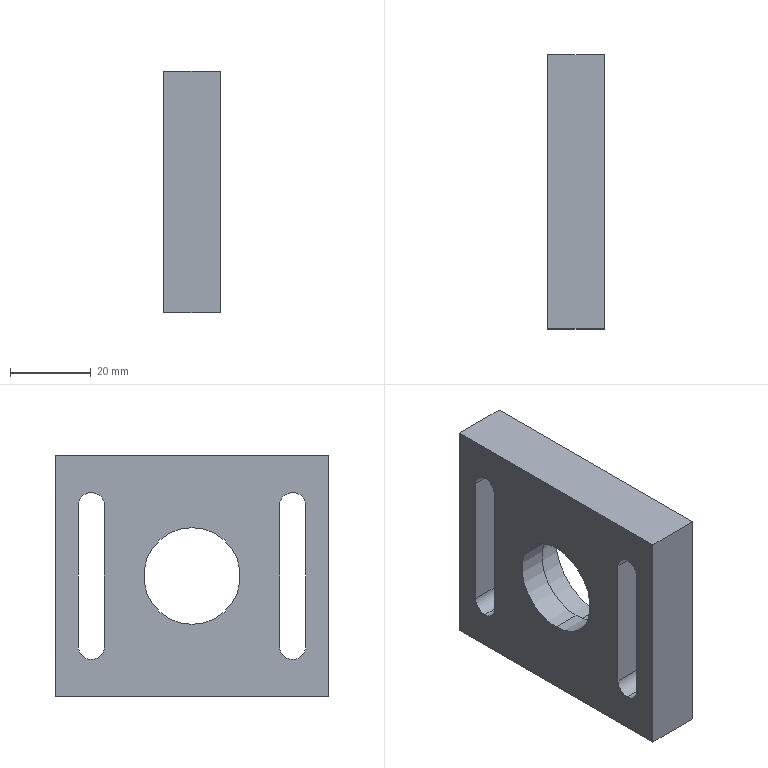Part | STEP file | PN_0033 (secondary rotating shaft seat) | 1 solid | 21 faces | box 14 x 68 x 60 mm | volume 42344 mm3 | plane 11 | cylinder 10 | commonest cylinder face diameters 6.5 x6 24 x2 28 x2